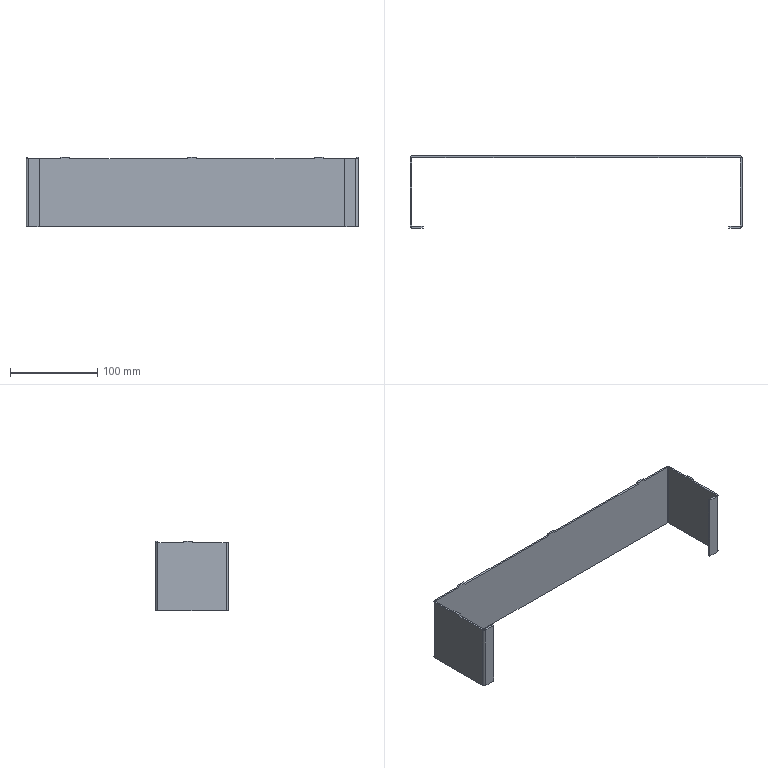Part | STEP file | xzz-003 | 1 solid | 42 faces | box 380 x 83 x 80 mm | volume 88406 mm3 | plane 34 | cylinder 8 | commonest cylinder face diameters 1 x4 5 x4
STEP:
#1=CARTESIAN_POINT('',(173.,20.,78.));
#2=VERTEX_POINT('',#1);
#3=CARTESIAN_POINT('',(210.5,20.,78.));
#4=VERTEX_POINT('',#3);
#5=CARTESIAN_POINT('',(-167.,20.,78.));
#6=DIRECTION('',(1.,0.,0.));
#7=VECTOR('',#6,1000.);
#8=LINE('',#5,#7);
#9=EDGE_CURVE('',#2,#4,#8,.T.);
#10=ORIENTED_EDGE('',*,*,#9,.T.);
#11=CARTESIAN_POINT('',(210.5,20.,0.));
#12=VERTEX_POINT('',#11);
#13=CARTESIAN_POINT('',(210.5,20.,78.));
#14=DIRECTION('',(0.,0.,-1.));
#15=VECTOR('',#14,1000.);
#16=LINE('',#13,#15);
#17=EDGE_CURVE('',#4,#12,#16,.T.);
#18=ORIENTED_EDGE('',*,*,#17,.T.);
#19=CARTESIAN_POINT('',(-164.5,20.,0.));
#20=VERTEX_POINT('',#19);
#21=CARTESIAN_POINT('',(-167.,20.,0.));
#22=DIRECTION('',(-1.,0.,0.));
#23=VECTOR('',#22,1000.);
#24=LINE('',#21,#23);
#25=EDGE_CURVE('',#12,#20,#24,.T.);
#26=ORIENTED_EDGE('',*,*,#25,.T.);
#27=CARTESIAN_POINT('',(-164.5,20.,78.));
#28=VERTEX_POINT('',#27);
#29=CARTESIAN_POINT('',(-164.5,20.,78.));
#30=DIRECTION('',(0.,0.,1.));
#31=VECTOR('',#30,1000.);
#32=LINE('',#29,#31);
#33=EDGE_CURVE('',#20,#28,#32,.T.);
#34=ORIENTED_EDGE('',*,*,#33,.T.);
#35=CARTESIAN_POINT('',(-127.,20.,78.));
#36=VERTEX_POINT('',#35);
#37=CARTESIAN_POINT('',(-167.,20.,78.));
#38=DIRECTION('',(1.,0.,0.));
#39=VECTOR('',#38,1000.);
#40=LINE('',#37,#39);
#41=EDGE_CURVE('',#28,#36,#40,.T.);
#42=ORIENTED_EDGE('',*,*,#41,.T.);
#43=CARTESIAN_POINT('',(-127.,20.,80.));
#44=VERTEX_POINT('',#43);
#45=CARTESIAN_POINT('',(-127.,20.,78.));
#46=DIRECTION('',(0.,0.,1.));
#47=VECTOR('',#46,1000.);
#48=LINE('',#45,#47);
#49=EDGE_CURVE('',#36,#44,#48,.T.);
#50=ORIENTED_EDGE('',*,*,#49,.T.);
#51=CARTESIAN_POINT('',(-117.,20.,80.));
#52=VERTEX_POINT('',#51);
#53=CARTESIAN_POINT('',(-167.,20.,80.));
#54=DIRECTION('',(1.,0.,0.));
#55=VECTOR('',#54,1000.);
#56=LINE('',#53,#55);
#57=EDGE_CURVE('',#44,#52,#56,.T.);
#58=ORIENTED_EDGE('',*,*,#57,.T.);
#59=CARTESIAN_POINT('',(-117.,20.,78.));
#60=VERTEX_POINT('',#59);
#61=CARTESIAN_POINT('',(-117.,20.,78.));
#62=DIRECTION('',(0.,0.,-1.));
#63=VECTOR('',#62,1000.);
#64=LINE('',#61,#63);
#65=EDGE_CURVE('',#52,#60,#64,.T.);
#66=ORIENTED_EDGE('',*,*,#65,.T.);
#67=CARTESIAN_POINT('',(18.,20.,78.));
#68=VERTEX_POINT('',#67);
#69=CARTESIAN_POINT('',(-167.,20.,78.));
#70=DIRECTION('',(1.,0.,0.));
#71=VECTOR('',#70,1000.);
#72=LINE('',#69,#71);
#73=EDGE_CURVE('',#60,#68,#72,.T.);
#74=ORIENTED_EDGE('',*,*,#73,.T.);
#75=CARTESIAN_POINT('',(18.,20.,80.));
#76=VERTEX_POINT('',#75);
#77=CARTESIAN_POINT('',(18.,20.,78.));
#78=DIRECTION('',(0.,0.,1.));
#79=VECTOR('',#78,1000.);
#80=LINE('',#77,#79);
#81=EDGE_CURVE('',#68,#76,#80,.T.);
#82=ORIENTED_EDGE('',*,*,#81,.T.);
#83=CARTESIAN_POINT('',(28.,20.,80.));
#84=VERTEX_POINT('',#83);
#85=CARTESIAN_POINT('',(-167.,20.,80.));
#86=DIRECTION('',(1.,0.,0.));
#87=VECTOR('',#86,1000.);
#88=LINE('',#85,#87);
#89=EDGE_CURVE('',#76,#84,#88,.T.);
#90=ORIENTED_EDGE('',*,*,#89,.T.);
#91=CARTESIAN_POINT('',(28.,20.,78.));
#92=VERTEX_POINT('',#91);
#93=CARTESIAN_POINT('',(28.,20.,78.));
#94=DIRECTION('',(0.,0.,-1.));
#95=VECTOR('',#94,1000.);
#96=LINE('',#93,#95);
#97=EDGE_CURVE('',#84,#92,#96,.T.);
#98=ORIENTED_EDGE('',*,*,#97,.T.);
#99=CARTESIAN_POINT('',(163.,20.,78.));
#100=VERTEX_POINT('',#99);
#101=CARTESIAN_POINT('',(-167.,20.,78.));
#102=DIRECTION('',(1.,0.,0.));
#103=VECTOR('',#102,1000.);
#104=LINE('',#101,#103);
#105=EDGE_CURVE('',#92,#100,#104,.T.);
#106=ORIENTED_EDGE('',*,*,#105,.T.);
#107=CARTESIAN_POINT('',(163.,20.,80.));
#108=VERTEX_POINT('',#107);
#109=CARTESIAN_POINT('',(163.,20.,78.));
#110=DIRECTION('',(0.,0.,1.));
#111=VECTOR('',#110,1000.);
#112=LINE('',#109,#111);
#113=EDGE_CURVE('',#100,#108,#112,.T.);
#114=ORIENTED_EDGE('',*,*,#113,.T.);
#115=CARTESIAN_POINT('',(173.,20.,80.));
#116=VERTEX_POINT('',#115);
#117=CARTESIAN_POINT('',(-167.,20.,80.));
#118=DIRECTION('',(1.,0.,0.));
#119=VECTOR('',#118,1000.);
#120=LINE('',#117,#119);
#121=EDGE_CURVE('',#108,#116,#120,.T.);
#122=ORIENTED_EDGE('',*,*,#121,.T.);
#123=CARTESIAN_POINT('',(173.,20.,78.));
#124=DIRECTION('',(0.,0.,-1.));
#125=VECTOR('',#124,1000.);
#126=LINE('',#123,#125);
#127=EDGE_CURVE('',#116,#2,#126,.T.);
#128=ORIENTED_EDGE('',*,*,#127,.T.);
#129=EDGE_LOOP('',(#10,#18,#26,#34,#42,#50,#58,#66,#74,#82,#90,#98,#106,#114,#122,#128));
#130=FACE_OUTER_BOUND('',#129,.T.);
#131=CARTESIAN_POINT('',(-167.,20.,78.));
#132=DIRECTION('',(0.,1.,0.));
#133=DIRECTION('',(0.,0.,1.));
#134=AXIS2_PLACEMENT_3D('',#131,#132,#133);
#135=PLANE('',#134);
#136=ADVANCED_FACE('',(#130),#135,.T.);
#137=CARTESIAN_POINT('',(213.,17.5,78.));
#138=VERTEX_POINT('',#137);
#139=CARTESIAN_POINT('',(210.5,17.5,78.));
#140=DIRECTION('',(0.,0.,-1.));
#141=DIRECTION('',(-1.,0.,0.));
#142=AXIS2_PLACEMENT_3D('',#139,#140,#141);
#143=CIRCLE('',#142,2.5);
#144=EDGE_CURVE('',#4,#138,#143,.T.);
#145=ORIENTED_EDGE('',*,*,#144,.T.);
#146=CARTESIAN_POINT('',(213.,17.5,0.));
#147=VERTEX_POINT('',#146);
#148=CARTESIAN_POINT('',(213.,17.5,78.));
#149=DIRECTION('',(0.,0.,-1.));
#150=VECTOR('',#149,1000.);
#151=LINE('',#148,#150);
#152=EDGE_CURVE('',#138,#147,#151,.T.);
#153=ORIENTED_EDGE('',*,*,#152,.T.);
#154=CARTESIAN_POINT('',(210.5,17.5,0.));
#155=DIRECTION('',(0.,0.,1.));
#156=DIRECTION('',(-1.,0.,0.));
#157=AXIS2_PLACEMENT_3D('',#154,#155,#156);
#158=CIRCLE('',#157,2.5);
#159=EDGE_CURVE('',#147,#12,#158,.T.);
#160=ORIENTED_EDGE('',*,*,#159,.T.);
#161=ORIENTED_EDGE('',*,*,#17,.F.);
#162=EDGE_LOOP('',(#145,#153,#160,#161));
#163=FACE_OUTER_BOUND('',#162,.T.);
#164=CARTESIAN_POINT('',(210.5,17.5,78.));
#165=DIRECTION('',(0.,0.,-1.));
#166=DIRECTION('',(-1.,0.,0.));
#167=AXIS2_PLACEMENT_3D('',#164,#165,#166);
#168=CYLINDRICAL_SURFACE('',#167,2.5);
#169=ADVANCED_FACE('',(#163),#168,.T.);
#170=CARTESIAN_POINT('',(173.,18.,78.));
#171=VERTEX_POINT('',#170);
#172=CARTESIAN_POINT('',(210.5,18.,78.));
#173=VERTEX_POINT('',#172);
#174=CARTESIAN_POINT('',(-165.,18.,78.));
#175=DIRECTION('',(1.,0.,0.));
#176=VECTOR('',#175,1000.);
#177=LINE('',#174,#176);
#178=EDGE_CURVE('',#171,#173,#177,.T.);
#179=ORIENTED_EDGE('',*,*,#178,.T.);
#180=CARTESIAN_POINT('',(211.,17.5,78.));
#181=VERTEX_POINT('',#180);
#182=CARTESIAN_POINT('',(210.5,17.5,78.));
#183=DIRECTION('',(0.,0.,-1.));
#184=DIRECTION('',(-1.,0.,0.));
#185=AXIS2_PLACEMENT_3D('',#182,#183,#184);
#186=CIRCLE('',#185,0.5);
#187=EDGE_CURVE('',#173,#181,#186,.T.);
#188=ORIENTED_EDGE('',*,*,#187,.T.);
#189=CARTESIAN_POINT('',(211.,-12.,78.));
#190=VERTEX_POINT('',#189);
#191=CARTESIAN_POINT('',(211.,18.,78.));
#192=DIRECTION('',(0.,-1.,0.));
#193=VECTOR('',#192,1000.);
#194=LINE('',#191,#193);
#195=EDGE_CURVE('',#181,#190,#194,.T.);
#196=ORIENTED_EDGE('',*,*,#195,.T.);
#197=CARTESIAN_POINT('',(213.,-12.,78.));
#198=VERTEX_POINT('',#197);
#199=CARTESIAN_POINT('',(213.,-12.,78.));
#200=DIRECTION('',(1.,0.,0.));
#201=VECTOR('',#200,1000.);
#202=LINE('',#199,#201);
#203=EDGE_CURVE('',#190,#198,#202,.T.);
#204=ORIENTED_EDGE('',*,*,#203,.T.);
#205=CARTESIAN_POINT('',(213.,20.,78.));
#206=DIRECTION('',(0.,-1.,0.));
#207=VECTOR('',#206,1000.);
#208=LINE('',#205,#207);
#209=EDGE_CURVE('',#138,#198,#208,.T.);
#210=ORIENTED_EDGE('',*,*,#209,.F.);
#211=ORIENTED_EDGE('',*,*,#144,.F.);
#212=ORIENTED_EDGE('',*,*,#9,.F.);
#213=CARTESIAN_POINT('',(173.,17.5,78.));
#214=DIRECTION('',(0.,-1.,0.));
#215=VECTOR('',#214,1000.);
#216=LINE('',#213,#215);
#217=EDGE_CURVE('',#2,#171,#216,.T.);
#218=ORIENTED_EDGE('',*,*,#217,.T.);
#219=EDGE_LOOP('',(#179,#188,#196,#204,#210,#211,#212,#218));
#220=FACE_OUTER_BOUND('',#219,.T.);
#221=CARTESIAN_POINT('',(-165.,17.5,78.));
#222=DIRECTION('',(0.,0.,1.));
#223=DIRECTION('',(1.,0.,0.));
#224=AXIS2_PLACEMENT_3D('',#221,#222,#223);
#225=PLANE('',#224);
#226=ADVANCED_FACE('',(#220),#225,.T.);
#227=ORIENTED_EDGE('',*,*,#127,.F.);
#228=CARTESIAN_POINT('',(173.,18.,80.));
#229=VERTEX_POINT('',#228);
#230=CARTESIAN_POINT('',(173.,20.,80.));
#231=DIRECTION('',(0.,1.,0.));
#232=VECTOR('',#231,1000.);
#233=LINE('',#230,#232);
#234=EDGE_CURVE('',#229,#116,#233,.T.);
#235=ORIENTED_EDGE('',*,*,#234,.F.);
#236=CARTESIAN_POINT('',(173.,18.,80.));
#237=DIRECTION('',(0.,0.,1.));
#238=VECTOR('',#237,1000.);
#239=LINE('',#236,#238);
#240=EDGE_CURVE('',#171,#229,#239,.T.);
#241=ORIENTED_EDGE('',*,*,#240,.F.);
#242=ORIENTED_EDGE('',*,*,#217,.F.);
#243=EDGE_LOOP('',(#227,#235,#241,#242));
#244=FACE_OUTER_BOUND('',#243,.T.);
#245=CARTESIAN_POINT('',(173.,20.,80.));
#246=DIRECTION('',(-1.,0.,0.));
#247=DIRECTION('',(0.,0.,1.));
#248=AXIS2_PLACEMENT_3D('',#245,#246,#247);
#249=PLANE('',#248);
#250=ADVANCED_FACE('',(#244),#249,.F.);
#251=CARTESIAN_POINT('',(163.,18.,80.));
#252=VERTEX_POINT('',#251);
#253=CARTESIAN_POINT('',(0.,18.,80.));
#254=DIRECTION('',(1.,0.,0.));
#255=VECTOR('',#254,1000.);
#256=LINE('',#253,#255);
#257=EDGE_CURVE('',#252,#229,#256,.T.);
#258=ORIENTED_EDGE('',*,*,#257,.T.);
#259=ORIENTED_EDGE('',*,*,#234,.T.);
#260=ORIENTED_EDGE('',*,*,#121,.F.);
#261=CARTESIAN_POINT('',(163.,0.,80.));
#262=DIRECTION('',(0.,-1.,0.));
#263=VECTOR('',#262,1000.);
#264=LINE('',#261,#263);
#265=EDGE_CURVE('',#108,#252,#264,.T.);
#266=ORIENTED_EDGE('',*,*,#265,.T.);
#267=EDGE_LOOP('',(#258,#259,#260,#266));
#268=FACE_OUTER_BOUND('',#267,.T.);
#269=CARTESIAN_POINT('',(0.,0.,80.));
#270=DIRECTION('',(0.,0.,1.));
#271=DIRECTION('',(1.,0.,0.));
#272=AXIS2_PLACEMENT_3D('',#269,#270,#271);
#273=PLANE('',#272);
#274=ADVANCED_FACE('',(#268),#273,.T.);
#275=CARTESIAN_POINT('',(163.,18.,78.));
#276=VERTEX_POINT('',#275);
#277=CARTESIAN_POINT('',(163.,18.,80.));
#278=DIRECTION('',(0.,0.,-1.));
#279=VECTOR('',#278,1000.);
#280=LINE('',#277,#279);
#281=EDGE_CURVE('',#252,#276,#280,.T.);
#282=ORIENTED_EDGE('',*,*,#281,.F.);
#283=ORIENTED_EDGE('',*,*,#265,.F.);
#284=ORIENTED_EDGE('',*,*,#113,.F.);
#285=CARTESIAN_POINT('',(163.,20.,78.));
#286=DIRECTION('',(0.,1.,0.));
#287=VECTOR('',#286,1000.);
#288=LINE('',#285,#287);
#289=EDGE_CURVE('',#276,#100,#288,.T.);
#290=ORIENTED_EDGE('',*,*,#289,.F.);
#291=EDGE_LOOP('',(#282,#283,#284,#290));
#292=FACE_OUTER_BOUND('',#291,.T.);
#293=CARTESIAN_POINT('',(163.,20.,80.));
#294=DIRECTION('',(1.,0.,0.));
#295=DIRECTION('',(0.,1.,0.));
#296=AXIS2_PLACEMENT_3D('',#293,#294,#295);
#297=PLANE('',#296);
#298=ADVANCED_FACE('',(#292),#297,.F.);
#299=ORIENTED_EDGE('',*,*,#105,.F.);
#300=CARTESIAN_POINT('',(28.,18.,78.));
#301=VERTEX_POINT('',#300);
#302=CARTESIAN_POINT('',(28.,17.5,78.));
#303=DIRECTION('',(0.,-1.,0.));
#304=VECTOR('',#303,1000.);
#305=LINE('',#302,#304);
#306=EDGE_CURVE('',#92,#301,#305,.T.);
#307=ORIENTED_EDGE('',*,*,#306,.T.);
#308=CARTESIAN_POINT('',(-165.,18.,78.));
#309=DIRECTION('',(1.,0.,0.));
#310=VECTOR('',#309,1000.);
#311=LINE('',#308,#310);
#312=EDGE_CURVE('',#301,#276,#311,.T.);
#313=ORIENTED_EDGE('',*,*,#312,.T.);
#314=ORIENTED_EDGE('',*,*,#289,.T.);
#315=EDGE_LOOP('',(#299,#307,#313,#314));
#316=FACE_OUTER_BOUND('',#315,.T.);
#317=CARTESIAN_POINT('',(-165.,17.5,78.));
#318=DIRECTION('',(0.,0.,1.));
#319=DIRECTION('',(1.,0.,0.));
#320=AXIS2_PLACEMENT_3D('',#317,#318,#319);
#321=PLANE('',#320);
#322=ADVANCED_FACE('',(#316),#321,.T.);
#323=ORIENTED_EDGE('',*,*,#97,.F.);
#324=CARTESIAN_POINT('',(28.,18.,80.));
#325=VERTEX_POINT('',#324);
#326=CARTESIAN_POINT('',(28.,20.,80.));
#327=DIRECTION('',(0.,1.,0.));
#328=VECTOR('',#327,1000.);
#329=LINE('',#326,#328);
#330=EDGE_CURVE('',#325,#84,#329,.T.);
#331=ORIENTED_EDGE('',*,*,#330,.F.);
#332=CARTESIAN_POINT('',(28.,18.,80.));
#333=DIRECTION('',(0.,0.,1.));
#334=VECTOR('',#333,1000.);
#335=LINE('',#332,#334);
#336=EDGE_CURVE('',#301,#325,#335,.T.);
#337=ORIENTED_EDGE('',*,*,#336,.F.);
#338=ORIENTED_EDGE('',*,*,#306,.F.);
#339=EDGE_LOOP('',(#323,#331,#337,#338));
#340=FACE_OUTER_BOUND('',#339,.T.);
#341=CARTESIAN_POINT('',(28.,20.,80.));
#342=DIRECTION('',(-1.,0.,0.));
#343=DIRECTION('',(0.,-1.,0.));
#344=AXIS2_PLACEMENT_3D('',#341,#342,#343);
#345=PLANE('',#344);
#346=ADVANCED_FACE('',(#340),#345,.F.);
#347=ORIENTED_EDGE('',*,*,#330,.T.);
#348=ORIENTED_EDGE('',*,*,#89,.F.);
#349=CARTESIAN_POINT('',(18.,18.,80.));
#350=VERTEX_POINT('',#349);
#351=CARTESIAN_POINT('',(18.,0.,80.));
#352=DIRECTION('',(0.,-1.,0.));
#353=VECTOR('',#352,1000.);
#354=LINE('',#351,#353);
#355=EDGE_CURVE('',#76,#350,#354,.T.);
#356=ORIENTED_EDGE('',*,*,#355,.T.);
#357=CARTESIAN_POINT('',(0.,18.,80.));
#358=DIRECTION('',(1.,0.,0.));
#359=VECTOR('',#358,1000.);
#360=LINE('',#357,#359);
#361=EDGE_CURVE('',#350,#325,#360,.T.);
#362=ORIENTED_EDGE('',*,*,#361,.T.);
#363=EDGE_LOOP('',(#347,#348,#356,#362));
#364=FACE_OUTER_BOUND('',#363,.T.);
#365=CARTESIAN_POINT('',(0.,0.,80.));
#366=DIRECTION('',(0.,0.,1.));
#367=DIRECTION('',(1.,0.,0.));
#368=AXIS2_PLACEMENT_3D('',#365,#366,#367);
#369=PLANE('',#368);
#370=ADVANCED_FACE('',(#364),#369,.T.);
#371=CARTESIAN_POINT('',(18.,18.,78.));
#372=VERTEX_POINT('',#371);
#373=CARTESIAN_POINT('',(18.,18.,80.));
#374=DIRECTION('',(0.,0.,-1.));
#375=VECTOR('',#374,1000.);
#376=LINE('',#373,#375);
#377=EDGE_CURVE('',#350,#372,#376,.T.);
#378=ORIENTED_EDGE('',*,*,#377,.F.);
#379=ORIENTED_EDGE('',*,*,#355,.F.);
#380=ORIENTED_EDGE('',*,*,#81,.F.);
#381=CARTESIAN_POINT('',(18.,20.,78.));
#382=DIRECTION('',(0.,1.,0.));
#383=VECTOR('',#382,1000.);
#384=LINE('',#381,#383);
#385=EDGE_CURVE('',#372,#68,#384,.T.);
#386=ORIENTED_EDGE('',*,*,#385,.F.);
#387=EDGE_LOOP('',(#378,#379,#380,#386));
#388=FACE_OUTER_BOUND('',#387,.T.);
#389=CARTESIAN_POINT('',(18.,20.,80.));
#390=DIRECTION('',(1.,0.,0.));
#391=DIRECTION('',(0.,1.,0.));
#392=AXIS2_PLACEMENT_3D('',#389,#390,#391);
#393=PLANE('',#392);
#394=ADVANCED_FACE('',(#388),#393,.F.);
#395=ORIENTED_EDGE('',*,*,#73,.F.);
#396=CARTESIAN_POINT('',(-117.,18.,78.));
#397=VERTEX_POINT('',#396);
#398=CARTESIAN_POINT('',(-117.,17.5,78.));
#399=DIRECTION('',(0.,-1.,0.));
#400=VECTOR('',#399,1000.);
#401=LINE('',#398,#400);
#402=EDGE_CURVE('',#60,#397,#401,.T.);
#403=ORIENTED_EDGE('',*,*,#402,.T.);
#404=CARTESIAN_POINT('',(-165.,18.,78.));
#405=DIRECTION('',(1.,0.,0.));
#406=VECTOR('',#405,1000.);
#407=LINE('',#404,#406);
#408=EDGE_CURVE('',#397,#372,#407,.T.);
#409=ORIENTED_EDGE('',*,*,#408,.T.);
#410=ORIENTED_EDGE('',*,*,#385,.T.);
#411=EDGE_LOOP('',(#395,#403,#409,#410));
#412=FACE_OUTER_BOUND('',#411,.T.);
#413=CARTESIAN_POINT('',(-165.,17.5,78.));
#414=DIRECTION('',(0.,0.,1.));
#415=DIRECTION('',(1.,0.,0.));
#416=AXIS2_PLACEMENT_3D('',#413,#414,#415);
#417=PLANE('',#416);
#418=ADVANCED_FACE('',(#412),#417,.T.);
#419=ORIENTED_EDGE('',*,*,#65,.F.);
#420=CARTESIAN_POINT('',(-117.,18.,80.));
#421=VERTEX_POINT('',#420);
#422=CARTESIAN_POINT('',(-117.,20.,80.));
#423=DIRECTION('',(0.,1.,0.));
#424=VECTOR('',#423,1000.);
#425=LINE('',#422,#424);
#426=EDGE_CURVE('',#421,#52,#425,.T.);
#427=ORIENTED_EDGE('',*,*,#426,.F.);
#428=CARTESIAN_POINT('',(-117.,18.,80.));
#429=DIRECTION('',(0.,0.,1.));
#430=VECTOR('',#429,1000.);
#431=LINE('',#428,#430);
#432=EDGE_CURVE('',#397,#421,#431,.T.);
#433=ORIENTED_EDGE('',*,*,#432,.F.);
#434=ORIENTED_EDGE('',*,*,#402,.F.);
#435=EDGE_LOOP('',(#419,#427,#433,#434));
#436=FACE_OUTER_BOUND('',#435,.T.);
#437=CARTESIAN_POINT('',(-117.,20.,80.));
#438=DIRECTION('',(-1.,0.,0.));
#439=DIRECTION('',(0.,-1.,0.));
#440=AXIS2_PLACEMENT_3D('',#437,#438,#439);
#441=PLANE('',#440);
#442=ADVANCED_FACE('',(#436),#441,.F.);
#443=ORIENTED_EDGE('',*,*,#426,.T.);
#444=ORIENTED_EDGE('',*,*,#57,.F.);
#445=CARTESIAN_POINT('',(-127.,18.,80.));
#446=VERTEX_POINT('',#445);
#447=CARTESIAN_POINT('',(-127.,0.,80.));
#448=DIRECTION('',(0.,-1.,0.));
#449=VECTOR('',#448,1000.);
#450=LINE('',#447,#449);
#451=EDGE_CURVE('',#44,#446,#450,.T.);
#452=ORIENTED_EDGE('',*,*,#451,.T.);
#453=CARTESIAN_POINT('',(0.,18.,80.));
#454=DIRECTION('',(1.,0.,0.));
#455=VECTOR('',#454,1000.);
#456=LINE('',#453,#455);
#457=EDGE_CURVE('',#446,#421,#456,.T.);
#458=ORIENTED_EDGE('',*,*,#457,.T.);
#459=EDGE_LOOP('',(#443,#444,#452,#458));
#460=FACE_OUTER_BOUND('',#459,.T.);
#461=CARTESIAN_POINT('',(0.,0.,80.));
#462=DIRECTION('',(0.,0.,1.));
#463=DIRECTION('',(1.,0.,0.));
#464=AXIS2_PLACEMENT_3D('',#461,#462,#463);
#465=PLANE('',#464);
#466=ADVANCED_FACE('',(#460),#465,.T.);
#467=CARTESIAN_POINT('',(-127.,18.,78.));
#468=VERTEX_POINT('',#467);
#469=CARTESIAN_POINT('',(-127.,18.,80.));
#470=DIRECTION('',(0.,0.,-1.));
#471=VECTOR('',#470,1000.);
#472=LINE('',#469,#471);
#473=EDGE_CURVE('',#446,#468,#472,.T.);
#474=ORIENTED_EDGE('',*,*,#473,.F.);
#475=ORIENTED_EDGE('',*,*,#451,.F.);
#476=ORIENTED_EDGE('',*,*,#49,.F.);
#477=CARTESIAN_POINT('',(-127.,20.,78.));
#478=DIRECTION('',(0.,1.,0.));
#479=VECTOR('',#478,1000.);
#480=LINE('',#477,#479);
#481=EDGE_CURVE('',#468,#36,#480,.T.);
#482=ORIENTED_EDGE('',*,*,#481,.F.);
#483=EDGE_LOOP('',(#474,#475,#476,#482));
#484=FACE_OUTER_BOUND('',#483,.T.);
#485=CARTESIAN_POINT('',(-127.,20.,80.));
#486=DIRECTION('',(1.,0.,0.));
#487=DIRECTION('',(0.,0.,-1.));
#488=AXIS2_PLACEMENT_3D('',#485,#486,#487);
#489=PLANE('',#488);
#490=ADVANCED_FACE('',(#484),#489,.F.);
#491=ORIENTED_EDGE('',*,*,#41,.F.);
#492=CARTESIAN_POINT('',(-167.,17.5,78.));
#493=VERTEX_POINT('',#492);
#494=CARTESIAN_POINT('',(-164.5,17.5,78.));
#495=DIRECTION('',(0.,0.,-1.));
#496=DIRECTION('',(-1.,0.,0.));
#497=AXIS2_PLACEMENT_3D('',#494,#495,#496);
#498=CIRCLE('',#497,2.5);
#499=EDGE_CURVE('',#493,#28,#498,.T.);
#500=ORIENTED_EDGE('',*,*,#499,.F.);
#501=CARTESIAN_POINT('',(-167.,-12.,78.));
#502=VERTEX_POINT('',#501);
#503=CARTESIAN_POINT('',(-167.,20.,78.));
#504=DIRECTION('',(0.,1.,0.));
#505=VECTOR('',#504,1000.);
#506=LINE('',#503,#505);
#507=EDGE_CURVE('',#502,#493,#506,.T.);
#508=ORIENTED_EDGE('',*,*,#507,.F.);
#509=CARTESIAN_POINT('',(-165.,-12.,78.));
#510=VERTEX_POINT('',#509);
#511=CARTESIAN_POINT('',(-164.5,-12.,78.));
#512=DIRECTION('',(1.,0.,0.));
#513=VECTOR('',#512,1000.);
#514=LINE('',#511,#513);
#515=EDGE_CURVE('',#502,#510,#514,.T.);
#516=ORIENTED_EDGE('',*,*,#515,.T.);
#517=CARTESIAN_POINT('',(-165.,17.5,78.));
#518=VERTEX_POINT('',#517);
#519=CARTESIAN_POINT('',(-165.,-61.,78.));
#520=DIRECTION('',(0.,1.,0.));
#521=VECTOR('',#520,1000.);
#522=LINE('',#519,#521);
#523=EDGE_CURVE('',#510,#518,#522,.T.);
#524=ORIENTED_EDGE('',*,*,#523,.T.);
#525=CARTESIAN_POINT('',(-164.5,18.,78.));
#526=VERTEX_POINT('',#525);
#527=CARTESIAN_POINT('',(-164.5,17.5,78.));
#528=DIRECTION('',(0.,0.,-1.));
#529=DIRECTION('',(-1.,0.,0.));
#530=AXIS2_PLACEMENT_3D('',#527,#528,#529);
#531=CIRCLE('',#530,0.5);
#532=EDGE_CURVE('',#518,#526,#531,.T.);
#533=ORIENTED_EDGE('',*,*,#532,.T.);
#534=CARTESIAN_POINT('',(-165.,18.,78.));
#535=DIRECTION('',(1.,0.,0.));
#536=VECTOR('',#535,1000.);
#537=LINE('',#534,#536);
#538=EDGE_CURVE('',#526,#468,#537,.T.);
#539=ORIENTED_EDGE('',*,*,#538,.T.);
#540=ORIENTED_EDGE('',*,*,#481,.T.);
#541=EDGE_LOOP('',(#491,#500,#508,#516,#524,#533,#539,#540));
#542=FACE_OUTER_BOUND('',#541,.T.);
#543=CARTESIAN_POINT('',(-165.,17.5,78.));
#544=DIRECTION('',(0.,0.,1.));
#545=DIRECTION('',(1.,0.,0.));
#546=AXIS2_PLACEMENT_3D('',#543,#544,#545);
#547=PLANE('',#546);
#548=ADVANCED_FACE('',(#542),#547,.T.);
#549=ORIENTED_EDGE('',*,*,#499,.T.);
#550=ORIENTED_EDGE('',*,*,#33,.F.);
#551=CARTESIAN_POINT('',(-167.,17.5,0.));
#552=VERTEX_POINT('',#551);
#553=CARTESIAN_POINT('',(-164.5,17.5,0.));
#554=DIRECTION('',(0.,0.,1.));
#555=DIRECTION('',(-1.,0.,0.));
#556=AXIS2_PLACEMENT_3D('',#553,#554,#555);
#557=CIRCLE('',#556,2.5);
#558=EDGE_CURVE('',#20,#552,#557,.T.);
#559=ORIENTED_EDGE('',*,*,#558,.T.);
#560=CARTESIAN_POINT('',(-167.,17.5,78.));
#561=DIRECTION('',(0.,0.,1.));
#562=VECTOR('',#561,1000.);
#563=LINE('',#560,#562);
#564=EDGE_CURVE('',#552,#493,#563,.T.);
#565=ORIENTED_EDGE('',*,*,#564,.T.);
#566=EDGE_LOOP('',(#549,#550,#559,#565));
#567=FACE_OUTER_BOUND('',#566,.T.);
#568=CARTESIAN_POINT('',(-164.5,17.5,78.));
#569=DIRECTION('',(0.,0.,-1.));
#570=DIRECTION('',(-1.,0.,0.));
#571=AXIS2_PLACEMENT_3D('',#568,#569,#570);
#572=CYLINDRICAL_SURFACE('',#571,2.5);
#573=ADVANCED_FACE('',(#567),#572,.T.);
#574=CARTESIAN_POINT('',(210.5,18.,0.));
#575=VERTEX_POINT('',#574);
#576=CARTESIAN_POINT('',(-164.5,18.,0.));
#577=VERTEX_POINT('',#576);
#578=CARTESIAN_POINT('',(211.,18.,0.));
#579=DIRECTION('',(-1.,0.,0.));
#580=VECTOR('',#579,1000.);
#581=LINE('',#578,#580);
#582=EDGE_CURVE('',#575,#577,#581,.T.);
#583=ORIENTED_EDGE('',*,*,#582,.T.);
#584=CARTESIAN_POINT('',(-165.,17.5,0.));
#585=VERTEX_POINT('',#584);
#586=CARTESIAN_POINT('',(-164.5,17.5,0.));
#587=DIRECTION('',(0.,0.,1.));
#588=DIRECTION('',(-1.,0.,0.));
#589=AXIS2_PLACEMENT_3D('',#586,#587,#588);
#590=CIRCLE('',#589,0.5);
#591=EDGE_CURVE('',#577,#585,#590,.T.);
#592=ORIENTED_EDGE('',*,*,#591,.T.);
#593=CARTESIAN_POINT('',(-165.,-60.5,0.));
#594=VERTEX_POINT('',#593);
#595=CARTESIAN_POINT('',(-165.,18.,0.));
#596=DIRECTION('',(0.,-1.,0.));
#597=VECTOR('',#596,1000.);
#598=LINE('',#595,#597);
#599=EDGE_CURVE('',#585,#594,#598,.T.);
#600=ORIENTED_EDGE('',*,*,#599,.T.);
#601=CARTESIAN_POINT('',(-164.5,-61.,0.));
#602=VERTEX_POINT('',#601);
#603=CARTESIAN_POINT('',(-164.5,-60.5,0.));
#604=DIRECTION('',(0.,0.,1.));
#605=DIRECTION('',(-1.,0.,0.));
#606=AXIS2_PLACEMENT_3D('',#603,#604,#605);
#607=CIRCLE('',#606,0.5);
#608=EDGE_CURVE('',#594,#602,#607,.T.);
#609=ORIENTED_EDGE('',*,*,#608,.T.);
#610=CARTESIAN_POINT('',(-152.,-61.,0.));
#611=VERTEX_POINT('',#610);
#612=CARTESIAN_POINT('',(-165.,-61.,0.));
#613=DIRECTION('',(1.,0.,0.));
#614=VECTOR('',#613,1000.);
#615=LINE('',#612,#614);
#616=EDGE_CURVE('',#602,#611,#615,.T.);
#617=ORIENTED_EDGE('',*,*,#616,.T.);
#618=CARTESIAN_POINT('',(-152.,-63.,0.));
#619=VERTEX_POINT('',#618);
#620=CARTESIAN_POINT('',(-152.,-61.,0.));
#621=DIRECTION('',(0.,1.,0.));
#622=VECTOR('',#621,1000.);
#623=LINE('',#620,#622);
#624=EDGE_CURVE('',#619,#611,#623,.T.);
#625=ORIENTED_EDGE('',*,*,#624,.F.);
#626=CARTESIAN_POINT('',(-164.5,-63.,0.));
#627=VERTEX_POINT('',#626);
#628=CARTESIAN_POINT('',(-167.,-63.,0.));
#629=DIRECTION('',(1.,0.,0.));
#630=VECTOR('',#629,1000.);
#631=LINE('',#628,#630);
#632=EDGE_CURVE('',#627,#619,#631,.T.);
#633=ORIENTED_EDGE('',*,*,#632,.F.);
#634=CARTESIAN_POINT('',(-167.,-60.5,0.));
#635=VERTEX_POINT('',#634);
#636=CARTESIAN_POINT('',(-164.5,-60.5,0.));
#637=DIRECTION('',(0.,0.,1.));
#638=DIRECTION('',(-1.,0.,0.));
#639=AXIS2_PLACEMENT_3D('',#636,#637,#638);
#640=CIRCLE('',#639,2.5);
#641=EDGE_CURVE('',#635,#627,#640,.T.);
#642=ORIENTED_EDGE('',*,*,#641,.F.);
#643=CARTESIAN_POINT('',(-167.,20.,0.));
#644=DIRECTION('',(0.,-1.,0.));
#645=VECTOR('',#644,1000.);
#646=LINE('',#643,#645);
#647=EDGE_CURVE('',#552,#635,#646,.T.);
#648=ORIENTED_EDGE('',*,*,#647,.F.);
#649=ORIENTED_EDGE('',*,*,#558,.F.);
#650=ORIENTED_EDGE('',*,*,#25,.F.);
#651=ORIENTED_EDGE('',*,*,#159,.F.);
#652=CARTESIAN_POINT('',(213.,-60.5,0.));
#653=VERTEX_POINT('',#652);
#654=CARTESIAN_POINT('',(213.,20.,0.));
#655=DIRECTION('',(0.,1.,0.));
#656=VECTOR('',#655,1000.);
#657=LINE('',#654,#656);
#658=EDGE_CURVE('',#653,#147,#657,.T.);
#659=ORIENTED_EDGE('',*,*,#658,.F.);
#660=CARTESIAN_POINT('',(210.5,-63.,0.));
#661=VERTEX_POINT('',#660);
#662=CARTESIAN_POINT('',(210.5,-60.5,0.));
#663=DIRECTION('',(0.,0.,1.));
#664=DIRECTION('',(-1.,0.,0.));
#665=AXIS2_PLACEMENT_3D('',#662,#663,#664);
#666=CIRCLE('',#665,2.5);
#667=EDGE_CURVE('',#661,#653,#666,.T.);
#668=ORIENTED_EDGE('',*,*,#667,.F.);
#669=CARTESIAN_POINT('',(198.,-63.,0.));
#670=VERTEX_POINT('',#669);
#671=CARTESIAN_POINT('',(213.,-63.,0.));
#672=DIRECTION('',(1.,0.,0.));
#673=VECTOR('',#672,1000.);
#674=LINE('',#671,#673);
#675=EDGE_CURVE('',#670,#661,#674,.T.);
#676=ORIENTED_EDGE('',*,*,#675,.F.);
#677=CARTESIAN_POINT('',(198.,-61.,0.));
#678=VERTEX_POINT('',#677);
#679=CARTESIAN_POINT('',(198.,-63.,0.));
#680=DIRECTION('',(0.,-1.,0.));
#681=VECTOR('',#680,1000.);
#682=LINE('',#679,#681);
#683=EDGE_CURVE('',#678,#670,#682,.T.);
#684=ORIENTED_EDGE('',*,*,#683,.F.);
#685=CARTESIAN_POINT('',(210.5,-61.,0.));
#686=VERTEX_POINT('',#685);
#687=CARTESIAN_POINT('',(210.5,-61.,0.));
#688=DIRECTION('',(-1.,0.,0.));
#689=VECTOR('',#688,1000.);
#690=LINE('',#687,#689);
#691=EDGE_CURVE('',#686,#678,#690,.T.);
#692=ORIENTED_EDGE('',*,*,#691,.F.);
#693=CARTESIAN_POINT('',(211.,-60.5,0.));
#694=VERTEX_POINT('',#693);
#695=CARTESIAN_POINT('',(210.5,-60.5,0.));
#696=DIRECTION('',(0.,0.,1.));
#697=DIRECTION('',(-1.,0.,0.));
#698=AXIS2_PLACEMENT_3D('',#695,#696,#697);
#699=CIRCLE('',#698,0.5);
#700=EDGE_CURVE('',#686,#694,#699,.T.);
#701=ORIENTED_EDGE('',*,*,#700,.T.);
#702=CARTESIAN_POINT('',(211.,17.5,0.));
#703=VERTEX_POINT('',#702);
#704=CARTESIAN_POINT('',(211.,-61.,0.));
#705=DIRECTION('',(0.,1.,0.));
#706=VECTOR('',#705,1000.);
#707=LINE('',#704,#706);
#708=EDGE_CURVE('',#694,#703,#707,.T.);
#709=ORIENTED_EDGE('',*,*,#708,.T.);
#710=CARTESIAN_POINT('',(210.5,17.5,0.));
#711=DIRECTION('',(0.,0.,1.));
#712=DIRECTION('',(-1.,0.,0.));
#713=AXIS2_PLACEMENT_3D('',#710,#711,#712);
#714=CIRCLE('',#713,0.5);
#715=EDGE_CURVE('',#703,#575,#714,.T.);
#716=ORIENTED_EDGE('',*,*,#715,.T.);
#717=EDGE_LOOP('',(#583,#592,#600,#609,#617,#625,#633,#642,#648,#649,#650,#651,#659,#668,#676,#684,#692,#701,#709,#716));
#718=FACE_OUTER_BOUND('',#717,.T.);
#719=CARTESIAN_POINT('',(211.,17.5,0.));
#720=DIRECTION('',(0.,0.,-1.));
#721=DIRECTION('',(-1.,0.,0.));
#722=AXIS2_PLACEMENT_3D('',#719,#720,#721);
#723=PLANE('',#722);
#724=ADVANCED_FACE('',(#718),#723,.T.);
#725=CARTESIAN_POINT('',(213.,-22.,78.));
#726=VERTEX_POINT('',#725);
#727=CARTESIAN_POINT('',(213.,-60.5,78.));
#728=VERTEX_POINT('',#727);
#729=CARTESIAN_POINT('',(213.,20.,78.));
#730=DIRECTION('',(0.,-1.,0.));
#731=VECTOR('',#730,1000.);
#732=LINE('',#729,#731);
#733=EDGE_CURVE('',#726,#728,#732,.T.);
#734=ORIENTED_EDGE('',*,*,#733,.T.);
#735=CARTESIAN_POINT('',(213.,-60.5,78.));
#736=DIRECTION('',(0.,0.,-1.));
#737=VECTOR('',#736,1000.);
#738=LINE('',#735,#737);
#739=EDGE_CURVE('',#728,#653,#738,.T.);
#740=ORIENTED_EDGE('',*,*,#739,.T.);
#741=ORIENTED_EDGE('',*,*,#658,.T.);
#742=ORIENTED_EDGE('',*,*,#152,.F.);
#743=ORIENTED_EDGE('',*,*,#209,.T.);
#744=CARTESIAN_POINT('',(213.,-12.,80.));
#745=VERTEX_POINT('',#744);
#746=CARTESIAN_POINT('',(213.,-12.,78.));
#747=DIRECTION('',(0.,0.,1.));
#748=VECTOR('',#747,1000.);
#749=LINE('',#746,#748);
#750=EDGE_CURVE('',#198,#745,#749,.T.);
#751=ORIENTED_EDGE('',*,*,#750,.T.);
#752=CARTESIAN_POINT('',(213.,-22.,80.));
#753=VERTEX_POINT('',#752);
#754=CARTESIAN_POINT('',(213.,20.,80.));
#755=DIRECTION('',(0.,-1.,0.));
#756=VECTOR('',#755,1000.);
#757=LINE('',#754,#756);
#758=EDGE_CURVE('',#745,#753,#757,.T.);
#759=ORIENTED_EDGE('',*,*,#758,.T.);
#760=CARTESIAN_POINT('',(213.,-22.,78.));
#761=DIRECTION('',(0.,0.,-1.));
#762=VECTOR('',#761,1000.);
#763=LINE('',#760,#762);
#764=EDGE_CURVE('',#753,#726,#763,.T.);
#765=ORIENTED_EDGE('',*,*,#764,.T.);
#766=EDGE_LOOP('',(#734,#740,#741,#742,#743,#751,#759,#765));
#767=FACE_OUTER_BOUND('',#766,.T.);
#768=CARTESIAN_POINT('',(213.,20.,78.));
#769=DIRECTION('',(1.,0.,0.));
#770=DIRECTION('',(0.,1.,0.));
#771=AXIS2_PLACEMENT_3D('',#768,#769,#770);
#772=PLANE('',#771);
#773=ADVANCED_FACE('',(#767),#772,.T.);
#774=CARTESIAN_POINT('',(210.5,18.,78.));
#775=DIRECTION('',(0.,0.,-1.));
#776=VECTOR('',#775,1000.);
#777=LINE('',#774,#776);
#778=EDGE_CURVE('',#173,#575,#777,.T.);
#779=ORIENTED_EDGE('',*,*,#778,.F.);
#780=ORIENTED_EDGE('',*,*,#178,.F.);
#781=ORIENTED_EDGE('',*,*,#240,.T.);
#782=ORIENTED_EDGE('',*,*,#257,.F.);
#783=ORIENTED_EDGE('',*,*,#281,.T.);
#784=ORIENTED_EDGE('',*,*,#312,.F.);
#785=ORIENTED_EDGE('',*,*,#336,.T.);
#786=ORIENTED_EDGE('',*,*,#361,.F.);
#787=ORIENTED_EDGE('',*,*,#377,.T.);
#788=ORIENTED_EDGE('',*,*,#408,.F.);
#789=ORIENTED_EDGE('',*,*,#432,.T.);
#790=ORIENTED_EDGE('',*,*,#457,.F.);
#791=ORIENTED_EDGE('',*,*,#473,.T.);
#792=ORIENTED_EDGE('',*,*,#538,.F.);
#793=CARTESIAN_POINT('',(-164.5,18.,78.));
#794=DIRECTION('',(0.,0.,1.));
#795=VECTOR('',#794,1000.);
#796=LINE('',#793,#795);
#797=EDGE_CURVE('',#577,#526,#796,.T.);
#798=ORIENTED_EDGE('',*,*,#797,.F.);
#799=ORIENTED_EDGE('',*,*,#582,.F.);
#800=EDGE_LOOP('',(#779,#780,#781,#782,#783,#784,#785,#786,#787,#788,#789,#790,#791,#792,#798,#799));
#801=FACE_OUTER_BOUND('',#800,.T.);
#802=CARTESIAN_POINT('',(-167.,18.,78.));
#803=DIRECTION('',(0.,1.,0.));
#804=DIRECTION('',(0.,0.,1.));
#805=AXIS2_PLACEMENT_3D('',#802,#803,#804);
#806=PLANE('',#805);
#807=ADVANCED_FACE('',(#801),#806,.F.);
#808=ORIENTED_EDGE('',*,*,#507,.T.);
#809=ORIENTED_EDGE('',*,*,#564,.F.);
#810=ORIENTED_EDGE('',*,*,#647,.T.);
#811=CARTESIAN_POINT('',(-167.,-60.5,78.));
#812=VERTEX_POINT('',#811);
#813=CARTESIAN_POINT('',(-167.,-60.5,78.));
#814=DIRECTION('',(0.,0.,1.));
#815=VECTOR('',#814,1000.);
#816=LINE('',#813,#815);
#817=EDGE_CURVE('',#635,#812,#816,.T.);
#818=ORIENTED_EDGE('',*,*,#817,.T.);
#819=CARTESIAN_POINT('',(-167.,-22.,78.));
#820=VERTEX_POINT('',#819);
#821=CARTESIAN_POINT('',(-167.,20.,78.));
#822=DIRECTION('',(0.,1.,0.));
#823=VECTOR('',#822,1000.);
#824=LINE('',#821,#823);
#825=EDGE_CURVE('',#812,#820,#824,.T.);
#826=ORIENTED_EDGE('',*,*,#825,.T.);
#827=CARTESIAN_POINT('',(-167.,-22.,80.));
#828=VERTEX_POINT('',#827);
#829=CARTESIAN_POINT('',(-167.,-22.,78.));
#830=DIRECTION('',(0.,0.,1.));
#831=VECTOR('',#830,1000.);
#832=LINE('',#829,#831);
#833=EDGE_CURVE('',#820,#828,#832,.T.);
#834=ORIENTED_EDGE('',*,*,#833,.T.);
#835=CARTESIAN_POINT('',(-167.,-12.,80.));
#836=VERTEX_POINT('',#835);
#837=CARTESIAN_POINT('',(-167.,20.,80.));
#838=DIRECTION('',(0.,1.,0.));
#839=VECTOR('',#838,1000.);
#840=LINE('',#837,#839);
#841=EDGE_CURVE('',#828,#836,#840,.T.);
#842=ORIENTED_EDGE('',*,*,#841,.T.);
#843=CARTESIAN_POINT('',(-167.,-12.,78.));
#844=DIRECTION('',(0.,0.,-1.));
#845=VECTOR('',#844,1000.);
#846=LINE('',#843,#845);
#847=EDGE_CURVE('',#836,#502,#846,.T.);
#848=ORIENTED_EDGE('',*,*,#847,.T.);
#849=EDGE_LOOP('',(#808,#809,#810,#818,#826,#834,#842,#848));
#850=FACE_OUTER_BOUND('',#849,.T.);
#851=CARTESIAN_POINT('',(-167.,20.,78.));
#852=DIRECTION('',(-1.,0.,0.));
#853=DIRECTION('',(0.,0.,1.));
#854=AXIS2_PLACEMENT_3D('',#851,#852,#853);
#855=PLANE('',#854);
#856=ADVANCED_FACE('',(#850),#855,.T.);
#857=CARTESIAN_POINT('',(210.5,-63.,78.));
#858=VERTEX_POINT('',#857);
#859=CARTESIAN_POINT('',(210.5,-60.5,78.));
#860=DIRECTION('',(0.,0.,-1.));
#861=DIRECTION('',(-1.,0.,0.));
#862=AXIS2_PLACEMENT_3D('',#859,#860,#861);
#863=CIRCLE('',#862,2.5);
#864=EDGE_CURVE('',#728,#858,#863,.T.);
#865=ORIENTED_EDGE('',*,*,#864,.T.);
#866=CARTESIAN_POINT('',(210.5,-63.,78.));
#867=DIRECTION('',(0.,0.,-1.));
#868=VECTOR('',#867,1000.);
#869=LINE('',#866,#868);
#870=EDGE_CURVE('',#858,#661,#869,.T.);
#871=ORIENTED_EDGE('',*,*,#870,.T.);
#872=ORIENTED_EDGE('',*,*,#667,.T.);
#873=ORIENTED_EDGE('',*,*,#739,.F.);
#874=EDGE_LOOP('',(#865,#871,#872,#873));
#875=FACE_OUTER_BOUND('',#874,.T.);
#876=CARTESIAN_POINT('',(210.5,-60.5,78.));
#877=DIRECTION('',(0.,0.,-1.));
#878=DIRECTION('',(-1.,0.,0.));
#879=AXIS2_PLACEMENT_3D('',#876,#877,#878);
#880=CYLINDRICAL_SURFACE('',#879,2.5);
#881=ADVANCED_FACE('',(#875),#880,.T.);
#882=CARTESIAN_POINT('',(211.,-22.,78.));
#883=VERTEX_POINT('',#882);
#884=CARTESIAN_POINT('',(211.,-60.5,78.));
#885=VERTEX_POINT('',#884);
#886=CARTESIAN_POINT('',(211.,18.,78.));
#887=DIRECTION('',(0.,-1.,0.));
#888=VECTOR('',#887,1000.);
#889=LINE('',#886,#888);
#890=EDGE_CURVE('',#883,#885,#889,.T.);
#891=ORIENTED_EDGE('',*,*,#890,.T.);
#892=CARTESIAN_POINT('',(210.5,-61.,78.));
#893=VERTEX_POINT('',#892);
#894=CARTESIAN_POINT('',(210.5,-60.5,78.));
#895=DIRECTION('',(0.,0.,-1.));
#896=DIRECTION('',(-1.,0.,0.));
#897=AXIS2_PLACEMENT_3D('',#894,#895,#896);
#898=CIRCLE('',#897,0.5);
#899=EDGE_CURVE('',#885,#893,#898,.T.);
#900=ORIENTED_EDGE('',*,*,#899,.T.);
#901=CARTESIAN_POINT('',(198.,-61.,78.));
#902=VERTEX_POINT('',#901);
#903=CARTESIAN_POINT('',(211.,-61.,78.));
#904=DIRECTION('',(-1.,0.,0.));
#905=VECTOR('',#904,1000.);
#906=LINE('',#903,#905);
#907=EDGE_CURVE('',#893,#902,#906,.T.);
#908=ORIENTED_EDGE('',*,*,#907,.T.);
#909=CARTESIAN_POINT('',(198.,-63.,78.));
#910=VERTEX_POINT('',#909);
#911=CARTESIAN_POINT('',(198.,-63.,78.));
#912=DIRECTION('',(0.,1.,0.));
#913=VECTOR('',#912,1000.);
#914=LINE('',#911,#913);
#915=EDGE_CURVE('',#910,#902,#914,.T.);
#916=ORIENTED_EDGE('',*,*,#915,.F.);
#917=CARTESIAN_POINT('',(213.,-63.,78.));
#918=DIRECTION('',(-1.,0.,0.));
#919=VECTOR('',#918,1000.);
#920=LINE('',#917,#919);
#921=EDGE_CURVE('',#858,#910,#920,.T.);
#922=ORIENTED_EDGE('',*,*,#921,.F.);
#923=ORIENTED_EDGE('',*,*,#864,.F.);
#924=ORIENTED_EDGE('',*,*,#733,.F.);
#925=CARTESIAN_POINT('',(210.5,-22.,78.));
#926=DIRECTION('',(-1.,0.,0.));
#927=VECTOR('',#926,1000.);
#928=LINE('',#925,#927);
#929=EDGE_CURVE('',#726,#883,#928,.T.);
#930=ORIENTED_EDGE('',*,*,#929,.T.);
#931=EDGE_LOOP('',(#891,#900,#908,#916,#922,#923,#924,#930));
#932=FACE_OUTER_BOUND('',#931,.T.);
#933=CARTESIAN_POINT('',(210.5,18.,78.));
#934=DIRECTION('',(0.,0.,1.));
#935=DIRECTION('',(1.,0.,0.));
#936=AXIS2_PLACEMENT_3D('',#933,#934,#935);
#937=PLANE('',#936);
#938=ADVANCED_FACE('',(#932),#937,.T.);
#939=ORIENTED_EDGE('',*,*,#764,.F.);
#940=CARTESIAN_POINT('',(211.,-22.,80.));
#941=VERTEX_POINT('',#940);
#942=CARTESIAN_POINT('',(213.,-22.,80.));
#943=DIRECTION('',(1.,0.,0.));
#944=VECTOR('',#943,1000.);
#945=LINE('',#942,#944);
#946=EDGE_CURVE('',#941,#753,#945,.T.);
#947=ORIENTED_EDGE('',*,*,#946,.F.);
#948=CARTESIAN_POINT('',(211.,-22.,80.));
#949=DIRECTION('',(0.,0.,1.));
#950=VECTOR('',#949,1000.);
#951=LINE('',#948,#950);
#952=EDGE_CURVE('',#883,#941,#951,.T.);
#953=ORIENTED_EDGE('',*,*,#952,.F.);
#954=ORIENTED_EDGE('',*,*,#929,.F.);
#955=EDGE_LOOP('',(#939,#947,#953,#954));
#956=FACE_OUTER_BOUND('',#955,.T.);
#957=CARTESIAN_POINT('',(213.,-22.,80.));
#958=DIRECTION('',(0.,1.,0.));
#959=DIRECTION('',(0.,0.,1.));
#960=AXIS2_PLACEMENT_3D('',#957,#958,#959);
#961=PLANE('',#960);
#962=ADVANCED_FACE('',(#956),#961,.F.);
#963=ORIENTED_EDGE('',*,*,#946,.T.);
#964=ORIENTED_EDGE('',*,*,#758,.F.);
#965=CARTESIAN_POINT('',(211.,-12.,80.));
#966=VERTEX_POINT('',#965);
#967=CARTESIAN_POINT('',(0.,-12.,80.));
#968=DIRECTION('',(-1.,0.,0.));
#969=VECTOR('',#968,1000.);
#970=LINE('',#967,#969);
#971=EDGE_CURVE('',#745,#966,#970,.T.);
#972=ORIENTED_EDGE('',*,*,#971,.T.);
#973=CARTESIAN_POINT('',(211.,0.,80.));
#974=DIRECTION('',(0.,-1.,0.));
#975=VECTOR('',#974,1000.);
#976=LINE('',#973,#975);
#977=EDGE_CURVE('',#966,#941,#976,.T.);
#978=ORIENTED_EDGE('',*,*,#977,.T.);
#979=EDGE_LOOP('',(#963,#964,#972,#978));
#980=FACE_OUTER_BOUND('',#979,.T.);
#981=CARTESIAN_POINT('',(0.,0.,80.));
#982=DIRECTION('',(0.,0.,1.));
#983=DIRECTION('',(1.,0.,0.));
#984=AXIS2_PLACEMENT_3D('',#981,#982,#983);
#985=PLANE('',#984);
#986=ADVANCED_FACE('',(#980),#985,.T.);
#987=CARTESIAN_POINT('',(211.,-12.,80.));
#988=DIRECTION('',(0.,0.,-1.));
#989=VECTOR('',#988,1000.);
#990=LINE('',#987,#989);
#991=EDGE_CURVE('',#966,#190,#990,.T.);
#992=ORIENTED_EDGE('',*,*,#991,.F.);
#993=ORIENTED_EDGE('',*,*,#971,.F.);
#994=ORIENTED_EDGE('',*,*,#750,.F.);
#995=ORIENTED_EDGE('',*,*,#203,.F.);
#996=EDGE_LOOP('',(#992,#993,#994,#995));
#997=FACE_OUTER_BOUND('',#996,.T.);
#998=CARTESIAN_POINT('',(213.,-12.,80.));
#999=DIRECTION('',(0.,-1.,0.));
#1000=DIRECTION('',(0.,0.,-1.));
#1001=AXIS2_PLACEMENT_3D('',#998,#999,#1000);
#1002=PLANE('',#1001);
#1003=ADVANCED_FACE('',(#997),#1002,.F.);
#1004=CARTESIAN_POINT('',(211.,17.5,78.));
#1005=DIRECTION('',(0.,0.,-1.));
#1006=VECTOR('',#1005,1000.);
#1007=LINE('',#1004,#1006);
#1008=EDGE_CURVE('',#181,#703,#1007,.T.);
#1009=ORIENTED_EDGE('',*,*,#1008,.F.);
#1010=ORIENTED_EDGE('',*,*,#187,.F.);
#1011=ORIENTED_EDGE('',*,*,#778,.T.);
#1012=ORIENTED_EDGE('',*,*,#715,.F.);
#1013=EDGE_LOOP('',(#1009,#1010,#1011,#1012));
#1014=FACE_OUTER_BOUND('',#1013,.T.);
#1015=CARTESIAN_POINT('',(210.5,17.5,78.));
#1016=DIRECTION('',(0.,0.,-1.));
#1017=DIRECTION('',(-1.,0.,0.));
#1018=AXIS2_PLACEMENT_3D('',#1015,#1016,#1017);
#1019=CYLINDRICAL_SURFACE('',#1018,0.5);
#1020=ADVANCED_FACE('',(#1014),#1019,.F.);
#1021=ORIENTED_EDGE('',*,*,#797,.T.);
#1022=ORIENTED_EDGE('',*,*,#532,.F.);
#1023=CARTESIAN_POINT('',(-165.,17.5,78.));
#1024=DIRECTION('',(0.,0.,1.));
#1025=VECTOR('',#1024,1000.);
#1026=LINE('',#1023,#1025);
#1027=EDGE_CURVE('',#585,#518,#1026,.T.);
#1028=ORIENTED_EDGE('',*,*,#1027,.F.);
#1029=ORIENTED_EDGE('',*,*,#591,.F.);
#1030=EDGE_LOOP('',(#1021,#1022,#1028,#1029));
#1031=FACE_OUTER_BOUND('',#1030,.T.);
#1032=CARTESIAN_POINT('',(-164.5,17.5,78.));
#1033=DIRECTION('',(0.,0.,-1.));
#1034=DIRECTION('',(-1.,0.,0.));
#1035=AXIS2_PLACEMENT_3D('',#1032,#1033,#1034);
#1036=CYLINDRICAL_SURFACE('',#1035,0.5);
#1037=ADVANCED_FACE('',(#1031),#1036,.F.);
#1038=ORIENTED_EDGE('',*,*,#847,.F.);
#1039=CARTESIAN_POINT('',(-165.,-12.,80.));
#1040=VERTEX_POINT('',#1039);
#1041=CARTESIAN_POINT('',(-167.,-12.,80.));
#1042=DIRECTION('',(-1.,0.,0.));
#1043=VECTOR('',#1042,1000.);
#1044=LINE('',#1041,#1043);
#1045=EDGE_CURVE('',#1040,#836,#1044,.T.);
#1046=ORIENTED_EDGE('',*,*,#1045,.F.);
#1047=CARTESIAN_POINT('',(-165.,-12.,80.));
#1048=DIRECTION('',(0.,0.,1.));
#1049=VECTOR('',#1048,1000.);
#1050=LINE('',#1047,#1049);
#1051=EDGE_CURVE('',#510,#1040,#1050,.T.);
#1052=ORIENTED_EDGE('',*,*,#1051,.F.);
#1053=ORIENTED_EDGE('',*,*,#515,.F.);
#1054=EDGE_LOOP('',(#1038,#1046,#1052,#1053));
#1055=FACE_OUTER_BOUND('',#1054,.T.);
#1056=CARTESIAN_POINT('',(-167.,-12.,80.));
#1057=DIRECTION('',(0.,-1.,0.));
#1058=DIRECTION('',(0.,0.,-1.));
#1059=AXIS2_PLACEMENT_3D('',#1056,#1057,#1058);
#1060=PLANE('',#1059);
#1061=ADVANCED_FACE('',(#1055),#1060,.F.);
#1062=CARTESIAN_POINT('',(-165.,-22.,80.));
#1063=VERTEX_POINT('',#1062);
#1064=CARTESIAN_POINT('',(-165.,0.,80.));
#1065=DIRECTION('',(0.,1.,0.));
#1066=VECTOR('',#1065,1000.);
#1067=LINE('',#1064,#1066);
#1068=EDGE_CURVE('',#1063,#1040,#1067,.T.);
#1069=ORIENTED_EDGE('',*,*,#1068,.T.);
#1070=ORIENTED_EDGE('',*,*,#1045,.T.);
#1071=ORIENTED_EDGE('',*,*,#841,.F.);
#1072=CARTESIAN_POINT('',(0.,-22.,80.));
#1073=DIRECTION('',(1.,0.,0.));
#1074=VECTOR('',#1073,1000.);
#1075=LINE('',#1072,#1074);
#1076=EDGE_CURVE('',#828,#1063,#1075,.T.);
#1077=ORIENTED_EDGE('',*,*,#1076,.T.);
#1078=EDGE_LOOP('',(#1069,#1070,#1071,#1077));
#1079=FACE_OUTER_BOUND('',#1078,.T.);
#1080=CARTESIAN_POINT('',(0.,0.,80.));
#1081=DIRECTION('',(0.,0.,1.));
#1082=DIRECTION('',(1.,0.,0.));
#1083=AXIS2_PLACEMENT_3D('',#1080,#1081,#1082);
#1084=PLANE('',#1083);
#1085=ADVANCED_FACE('',(#1079),#1084,.T.);
#1086=CARTESIAN_POINT('',(-165.,-22.,78.));
#1087=VERTEX_POINT('',#1086);
#1088=CARTESIAN_POINT('',(-165.,-22.,80.));
#1089=DIRECTION('',(0.,0.,-1.));
#1090=VECTOR('',#1089,1000.);
#1091=LINE('',#1088,#1090);
#1092=EDGE_CURVE('',#1063,#1087,#1091,.T.);
#1093=ORIENTED_EDGE('',*,*,#1092,.F.);
#1094=ORIENTED_EDGE('',*,*,#1076,.F.);
#1095=ORIENTED_EDGE('',*,*,#833,.F.);
#1096=CARTESIAN_POINT('',(-167.,-22.,78.));
#1097=DIRECTION('',(-1.,0.,0.));
#1098=VECTOR('',#1097,1000.);
#1099=LINE('',#1096,#1098);
#1100=EDGE_CURVE('',#1087,#820,#1099,.T.);
#1101=ORIENTED_EDGE('',*,*,#1100,.F.);
#1102=EDGE_LOOP('',(#1093,#1094,#1095,#1101));
#1103=FACE_OUTER_BOUND('',#1102,.T.);
#1104=CARTESIAN_POINT('',(-167.,-22.,80.));
#1105=DIRECTION('',(0.,1.,0.));
#1106=DIRECTION('',(0.,0.,1.));
#1107=AXIS2_PLACEMENT_3D('',#1104,#1105,#1106);
#1108=PLANE('',#1107);
#1109=ADVANCED_FACE('',(#1103),#1108,.F.);
#1110=ORIENTED_EDGE('',*,*,#825,.F.);
#1111=CARTESIAN_POINT('',(-164.5,-63.,78.));
#1112=VERTEX_POINT('',#1111);
#1113=CARTESIAN_POINT('',(-164.5,-60.5,78.));
#1114=DIRECTION('',(0.,0.,-1.));
#1115=DIRECTION('',(-1.,0.,0.));
#1116=AXIS2_PLACEMENT_3D('',#1113,#1114,#1115);
#1117=CIRCLE('',#1116,2.5);
#1118=EDGE_CURVE('',#1112,#812,#1117,.T.);
#1119=ORIENTED_EDGE('',*,*,#1118,.F.);
#1120=CARTESIAN_POINT('',(-152.,-63.,78.));
#1121=VERTEX_POINT('',#1120);
#1122=CARTESIAN_POINT('',(-167.,-63.,78.));
#1123=DIRECTION('',(-1.,0.,0.));
#1124=VECTOR('',#1123,1000.);
#1125=LINE('',#1122,#1124);
#1126=EDGE_CURVE('',#1121,#1112,#1125,.T.);
#1127=ORIENTED_EDGE('',*,*,#1126,.F.);
#1128=CARTESIAN_POINT('',(-152.,-61.,78.));
#1129=VERTEX_POINT('',#1128);
#1130=CARTESIAN_POINT('',(-152.,-60.5,78.));
#1131=DIRECTION('',(0.,1.,0.));
#1132=VECTOR('',#1131,1000.);
#1133=LINE('',#1130,#1132);
#1134=EDGE_CURVE('',#1121,#1129,#1133,.T.);
#1135=ORIENTED_EDGE('',*,*,#1134,.T.);
#1136=CARTESIAN_POINT('',(-164.5,-61.,78.));
#1137=VERTEX_POINT('',#1136);
#1138=CARTESIAN_POINT('',(210.5,-61.,78.));
#1139=DIRECTION('',(-1.,0.,0.));
#1140=VECTOR('',#1139,1000.);
#1141=LINE('',#1138,#1140);
#1142=EDGE_CURVE('',#1129,#1137,#1141,.T.);
#1143=ORIENTED_EDGE('',*,*,#1142,.T.);
#1144=CARTESIAN_POINT('',(-165.,-60.5,78.));
#1145=VERTEX_POINT('',#1144);
#1146=CARTESIAN_POINT('',(-164.5,-60.5,78.));
#1147=DIRECTION('',(0.,0.,-1.));
#1148=DIRECTION('',(-1.,0.,0.));
#1149=AXIS2_PLACEMENT_3D('',#1146,#1147,#1148);
#1150=CIRCLE('',#1149,0.5);
#1151=EDGE_CURVE('',#1137,#1145,#1150,.T.);
#1152=ORIENTED_EDGE('',*,*,#1151,.T.);
#1153=CARTESIAN_POINT('',(-165.,-61.,78.));
#1154=DIRECTION('',(0.,1.,0.));
#1155=VECTOR('',#1154,1000.);
#1156=LINE('',#1153,#1155);
#1157=EDGE_CURVE('',#1145,#1087,#1156,.T.);
#1158=ORIENTED_EDGE('',*,*,#1157,.T.);
#1159=ORIENTED_EDGE('',*,*,#1100,.T.);
#1160=EDGE_LOOP('',(#1110,#1119,#1127,#1135,#1143,#1152,#1158,#1159));
#1161=FACE_OUTER_BOUND('',#1160,.T.);
#1162=CARTESIAN_POINT('',(-164.5,-61.,78.));
#1163=DIRECTION('',(0.,0.,1.));
#1164=DIRECTION('',(1.,0.,0.));
#1165=AXIS2_PLACEMENT_3D('',#1162,#1163,#1164);
#1166=PLANE('',#1165);
#1167=ADVANCED_FACE('',(#1161),#1166,.T.);
#1168=ORIENTED_EDGE('',*,*,#1118,.T.);
#1169=ORIENTED_EDGE('',*,*,#817,.F.);
#1170=ORIENTED_EDGE('',*,*,#641,.T.);
#1171=CARTESIAN_POINT('',(-164.5,-63.,78.));
#1172=DIRECTION('',(0.,0.,1.));
#1173=VECTOR('',#1172,1000.);
#1174=LINE('',#1171,#1173);
#1175=EDGE_CURVE('',#627,#1112,#1174,.T.);
#1176=ORIENTED_EDGE('',*,*,#1175,.T.);
#1177=EDGE_LOOP('',(#1168,#1169,#1170,#1176));
#1178=FACE_OUTER_BOUND('',#1177,.T.);
#1179=CARTESIAN_POINT('',(-164.5,-60.5,78.));
#1180=DIRECTION('',(0.,0.,-1.));
#1181=DIRECTION('',(-1.,0.,0.));
#1182=AXIS2_PLACEMENT_3D('',#1179,#1180,#1181);
#1183=CYLINDRICAL_SURFACE('',#1182,2.5);
#1184=ADVANCED_FACE('',(#1178),#1183,.T.);
#1185=ORIENTED_EDGE('',*,*,#921,.T.);
#1186=CARTESIAN_POINT('',(198.,-63.,78.));
#1187=DIRECTION('',(0.,0.,-1.));
#1188=VECTOR('',#1187,1000.);
#1189=LINE('',#1186,#1188);
#1190=EDGE_CURVE('',#910,#670,#1189,.T.);
#1191=ORIENTED_EDGE('',*,*,#1190,.T.);
#1192=ORIENTED_EDGE('',*,*,#675,.T.);
#1193=ORIENTED_EDGE('',*,*,#870,.F.);
#1194=EDGE_LOOP('',(#1185,#1191,#1192,#1193));
#1195=FACE_OUTER_BOUND('',#1194,.T.);
#1196=CARTESIAN_POINT('',(213.,-63.,78.));
#1197=DIRECTION('',(0.,-1.,0.));
#1198=DIRECTION('',(0.,0.,-1.));
#1199=AXIS2_PLACEMENT_3D('',#1196,#1197,#1198);
#1200=PLANE('',#1199);
#1201=ADVANCED_FACE('',(#1195),#1200,.T.);
#1202=CARTESIAN_POINT('',(211.,-60.5,78.));
#1203=DIRECTION('',(0.,0.,-1.));
#1204=VECTOR('',#1203,1000.);
#1205=LINE('',#1202,#1204);
#1206=EDGE_CURVE('',#885,#694,#1205,.T.);
#1207=ORIENTED_EDGE('',*,*,#1206,.F.);
#1208=ORIENTED_EDGE('',*,*,#890,.F.);
#1209=ORIENTED_EDGE('',*,*,#952,.T.);
#1210=ORIENTED_EDGE('',*,*,#977,.F.);
#1211=ORIENTED_EDGE('',*,*,#991,.T.);
#1212=ORIENTED_EDGE('',*,*,#195,.F.);
#1213=ORIENTED_EDGE('',*,*,#1008,.T.);
#1214=ORIENTED_EDGE('',*,*,#708,.F.);
#1215=EDGE_LOOP('',(#1207,#1208,#1209,#1210,#1211,#1212,#1213,#1214));
#1216=FACE_OUTER_BOUND('',#1215,.T.);
#1217=CARTESIAN_POINT('',(211.,20.,78.));
#1218=DIRECTION('',(1.,0.,0.));
#1219=DIRECTION('',(0.,1.,0.));
#1220=AXIS2_PLACEMENT_3D('',#1217,#1218,#1219);
#1221=PLANE('',#1220);
#1222=ADVANCED_FACE('',(#1216),#1221,.F.);
#1223=ORIENTED_EDGE('',*,*,#1027,.T.);
#1224=ORIENTED_EDGE('',*,*,#523,.F.);
#1225=ORIENTED_EDGE('',*,*,#1051,.T.);
#1226=ORIENTED_EDGE('',*,*,#1068,.F.);
#1227=ORIENTED_EDGE('',*,*,#1092,.T.);
#1228=ORIENTED_EDGE('',*,*,#1157,.F.);
#1229=CARTESIAN_POINT('',(-165.,-60.5,78.));
#1230=DIRECTION('',(0.,0.,1.));
#1231=VECTOR('',#1230,1000.);
#1232=LINE('',#1229,#1231);
#1233=EDGE_CURVE('',#594,#1145,#1232,.T.);
#1234=ORIENTED_EDGE('',*,*,#1233,.F.);
#1235=ORIENTED_EDGE('',*,*,#599,.F.);
#1236=EDGE_LOOP('',(#1223,#1224,#1225,#1226,#1227,#1228,#1234,#1235));
#1237=FACE_OUTER_BOUND('',#1236,.T.);
#1238=CARTESIAN_POINT('',(-165.,20.,78.));
#1239=DIRECTION('',(-1.,0.,0.));
#1240=DIRECTION('',(0.,0.,1.));
#1241=AXIS2_PLACEMENT_3D('',#1238,#1239,#1240);
#1242=PLANE('',#1241);
#1243=ADVANCED_FACE('',(#1237),#1242,.F.);
#1244=ORIENTED_EDGE('',*,*,#1126,.T.);
#1245=ORIENTED_EDGE('',*,*,#1175,.F.);
#1246=ORIENTED_EDGE('',*,*,#632,.T.);
#1247=CARTESIAN_POINT('',(-152.,-63.,78.));
#1248=DIRECTION('',(0.,0.,1.));
#1249=VECTOR('',#1248,1000.);
#1250=LINE('',#1247,#1249);
#1251=EDGE_CURVE('',#619,#1121,#1250,.T.);
#1252=ORIENTED_EDGE('',*,*,#1251,.T.);
#1253=EDGE_LOOP('',(#1244,#1245,#1246,#1252));
#1254=FACE_OUTER_BOUND('',#1253,.T.);
#1255=CARTESIAN_POINT('',(-167.,-63.,78.));
#1256=DIRECTION('',(0.,-1.,0.));
#1257=DIRECTION('',(0.,0.,-1.));
#1258=AXIS2_PLACEMENT_3D('',#1255,#1256,#1257);
#1259=PLANE('',#1258);
#1260=ADVANCED_FACE('',(#1254),#1259,.T.);
#1261=ORIENTED_EDGE('',*,*,#915,.T.);
#1262=CARTESIAN_POINT('',(198.,-61.,78.));
#1263=DIRECTION('',(0.,0.,-1.));
#1264=VECTOR('',#1263,1000.);
#1265=LINE('',#1262,#1264);
#1266=EDGE_CURVE('',#902,#678,#1265,.T.);
#1267=ORIENTED_EDGE('',*,*,#1266,.T.);
#1268=ORIENTED_EDGE('',*,*,#683,.T.);
#1269=ORIENTED_EDGE('',*,*,#1190,.F.);
#1270=EDGE_LOOP('',(#1261,#1267,#1268,#1269));
#1271=FACE_OUTER_BOUND('',#1270,.T.);
#1272=CARTESIAN_POINT('',(198.,-63.,78.));
#1273=DIRECTION('',(-1.,0.,0.));
#1274=DIRECTION('',(0.,0.,1.));
#1275=AXIS2_PLACEMENT_3D('',#1272,#1273,#1274);
#1276=PLANE('',#1275);
#1277=ADVANCED_FACE('',(#1271),#1276,.T.);
#1278=CARTESIAN_POINT('',(210.5,-61.,78.));
#1279=DIRECTION('',(0.,0.,-1.));
#1280=VECTOR('',#1279,1000.);
#1281=LINE('',#1278,#1280);
#1282=EDGE_CURVE('',#893,#686,#1281,.T.);
#1283=ORIENTED_EDGE('',*,*,#1282,.F.);
#1284=ORIENTED_EDGE('',*,*,#899,.F.);
#1285=ORIENTED_EDGE('',*,*,#1206,.T.);
#1286=ORIENTED_EDGE('',*,*,#700,.F.);
#1287=EDGE_LOOP('',(#1283,#1284,#1285,#1286));
#1288=FACE_OUTER_BOUND('',#1287,.T.);
#1289=CARTESIAN_POINT('',(210.5,-60.5,78.));
#1290=DIRECTION('',(0.,0.,-1.));
#1291=DIRECTION('',(-1.,0.,0.));
#1292=AXIS2_PLACEMENT_3D('',#1289,#1290,#1291);
#1293=CYLINDRICAL_SURFACE('',#1292,0.5);
#1294=ADVANCED_FACE('',(#1288),#1293,.F.);
#1295=ORIENTED_EDGE('',*,*,#1233,.T.);
#1296=ORIENTED_EDGE('',*,*,#1151,.F.);
#1297=CARTESIAN_POINT('',(-164.5,-61.,78.));
#1298=DIRECTION('',(0.,0.,1.));
#1299=VECTOR('',#1298,1000.);
#1300=LINE('',#1297,#1299);
#1301=EDGE_CURVE('',#602,#1137,#1300,.T.);
#1302=ORIENTED_EDGE('',*,*,#1301,.F.);
#1303=ORIENTED_EDGE('',*,*,#608,.F.);
#1304=EDGE_LOOP('',(#1295,#1296,#1302,#1303));
#1305=FACE_OUTER_BOUND('',#1304,.T.);
#1306=CARTESIAN_POINT('',(-164.5,-60.5,78.));
#1307=DIRECTION('',(0.,0.,-1.));
#1308=DIRECTION('',(-1.,0.,0.));
#1309=AXIS2_PLACEMENT_3D('',#1306,#1307,#1308);
#1310=CYLINDRICAL_SURFACE('',#1309,0.5);
#1311=ADVANCED_FACE('',(#1305),#1310,.F.);
#1312=ORIENTED_EDGE('',*,*,#1134,.F.);
#1313=ORIENTED_EDGE('',*,*,#1251,.F.);
#1314=ORIENTED_EDGE('',*,*,#624,.T.);
#1315=CARTESIAN_POINT('',(-152.,-61.,78.));
#1316=DIRECTION('',(0.,0.,1.));
#1317=VECTOR('',#1316,1000.);
#1318=LINE('',#1315,#1317);
#1319=EDGE_CURVE('',#611,#1129,#1318,.T.);
#1320=ORIENTED_EDGE('',*,*,#1319,.T.);
#1321=EDGE_LOOP('',(#1312,#1313,#1314,#1320));
#1322=FACE_OUTER_BOUND('',#1321,.T.);
#1323=CARTESIAN_POINT('',(-152.,-61.,78.));
#1324=DIRECTION('',(1.,0.,0.));
#1325=DIRECTION('',(0.,0.,-1.));
#1326=AXIS2_PLACEMENT_3D('',#1323,#1324,#1325);
#1327=PLANE('',#1326);
#1328=ADVANCED_FACE('',(#1322),#1327,.T.);
#1329=ORIENTED_EDGE('',*,*,#1266,.F.);
#1330=ORIENTED_EDGE('',*,*,#907,.F.);
#1331=ORIENTED_EDGE('',*,*,#1282,.T.);
#1332=ORIENTED_EDGE('',*,*,#691,.T.);
#1333=EDGE_LOOP('',(#1329,#1330,#1331,#1332));
#1334=FACE_OUTER_BOUND('',#1333,.T.);
#1335=CARTESIAN_POINT('',(213.,-61.,78.));
#1336=DIRECTION('',(0.,-1.,0.));
#1337=DIRECTION('',(0.,0.,-1.));
#1338=AXIS2_PLACEMENT_3D('',#1335,#1336,#1337);
#1339=PLANE('',#1338);
#1340=ADVANCED_FACE('',(#1334),#1339,.F.);
#1341=ORIENTED_EDGE('',*,*,#1301,.T.);
#1342=ORIENTED_EDGE('',*,*,#1142,.F.);
#1343=ORIENTED_EDGE('',*,*,#1319,.F.);
#1344=ORIENTED_EDGE('',*,*,#616,.F.);
#1345=EDGE_LOOP('',(#1341,#1342,#1343,#1344));
#1346=FACE_OUTER_BOUND('',#1345,.T.);
#1347=CARTESIAN_POINT('',(-167.,-61.,78.));
#1348=DIRECTION('',(0.,-1.,0.));
#1349=DIRECTION('',(0.,0.,-1.));
#1350=AXIS2_PLACEMENT_3D('',#1347,#1348,#1349);
#1351=PLANE('',#1350);
#1352=ADVANCED_FACE('',(#1346),#1351,.F.);
#1353=CLOSED_SHELL('',(#136,#169,#226,#250,#274,#298,#322,#346,#370,#394,#418,#442,#466,#490,#548,#573,#724,#773,#807,#856,#881,#938,#962,#986,#1003,#1020,#1037,#1061,#1085,#1109,#1167,#1184,#1201,#1222,#1243,#1260,#1277,#1294,#1311,#1328,#1340,#1352));
#1354=MANIFOLD_SOLID_BREP('',#1353);
#1355=CARTESIAN_POINT('',(0.,0.,0.));
#1356=DIRECTION('',(0.,0.,1.));
#1357=DIRECTION('',(1.,0.,0.));
#1358=AXIS2_PLACEMENT_3D('',#1355,#1356,#1357);
#1359=(LENGTH_UNIT()NAMED_UNIT(*)SI_UNIT(.MILLI.,.METRE.));
#1360=UNCERTAINTY_MEASURE_WITH_UNIT(LENGTH_MEASURE(0.00001),#1359,'','');
#1361=(NAMED_UNIT(*)PLANE_ANGLE_UNIT()SI_UNIT($,.RADIAN.));
#1362=(NAMED_UNIT(*)SI_UNIT($,.STERADIAN.)SOLID_ANGLE_UNIT());
#1363=(GEOMETRIC_REPRESENTATION_CONTEXT(3)GLOBAL_UNCERTAINTY_ASSIGNED_CONTEXT((#1360))GLOBAL_UNIT_ASSIGNED_CONTEXT((#1359,#1361,#1362))REPRESENTATION_CONTEXT('',''));
#1364=ADVANCED_BREP_SHAPE_REPRESENTATION('',(#1354,#1358),#1363);